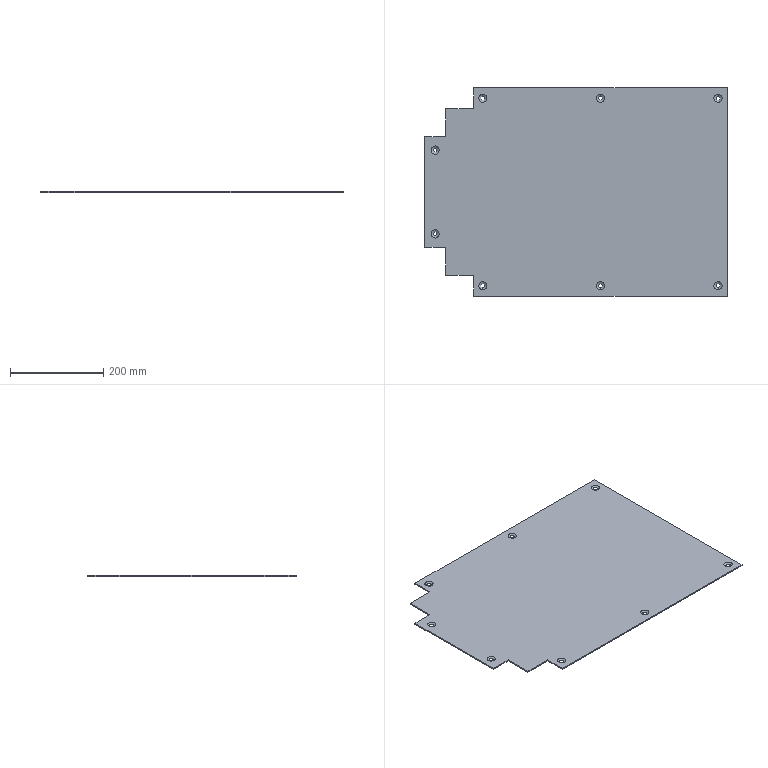Part | STEP file | PC rack top (asm 3) | 1 solid | 46 faces | box 650 x 448 x 2.5 mm | volume 688011 mm3 | cylinder 16 | cone 16 | plane 14 | commonest cylinder face diameters 9 x16